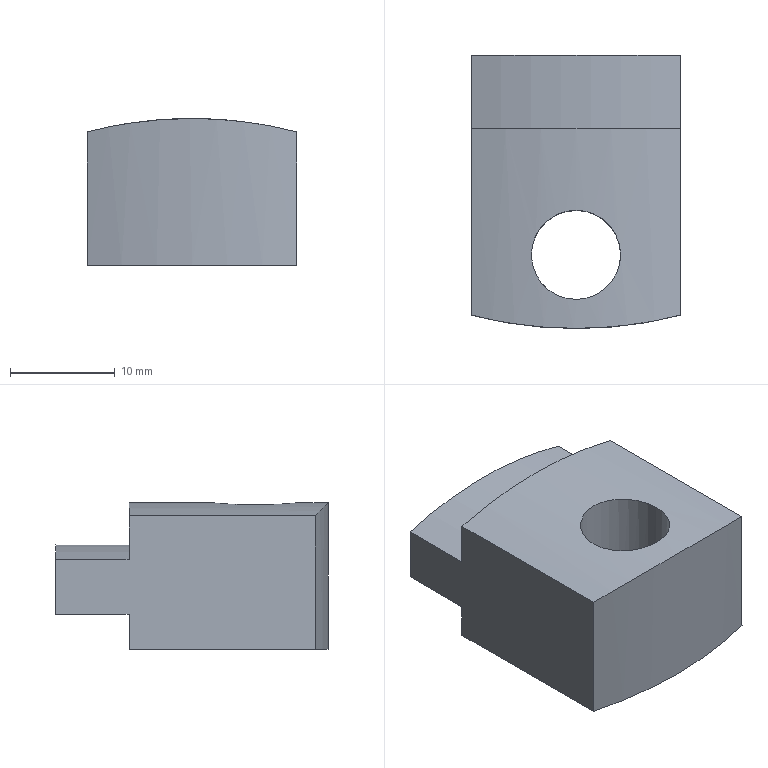Part | NX | features DATUM_CSYS 4, EXTRUDE 3, SKETCH 3 | 1 solid | 11 faces | box 20 x 26 x 14 mm | volume 4969 mm3 | plane 6 | cylinder 5 | commonest cylinder face diameters 80 x2 8.5 x1 62 x1 72 x1
STEP:
#1=CARTESIAN_POINT('',(10.,-21.,-3.657));
#2=VERTEX_POINT('',#1);
#3=CARTESIAN_POINT('',(-10.,-21.,-3.657));
#4=VERTEX_POINT('',#3);
#5=CARTESIAN_POINT('',(0.,-21.,-33.));
#6=DIRECTION('',(0.,-1.,0.));
#7=DIRECTION('',(-1.,0.,0.));
#8=AXIS2_PLACEMENT_3D('',#5,#6,#7);
#9=CIRCLE('',#8,31.);
#10=EDGE_CURVE('',#2,#4,#9,.T.);
#11=ORIENTED_EDGE('',*,*,#10,.F.);
#12=CARTESIAN_POINT('',(10.,-21.,-7.));
#13=VERTEX_POINT('',#12);
#14=CARTESIAN_POINT('',(10.,-21.,7.));
#15=DIRECTION('',(0.,0.,-1.));
#16=VECTOR('',#15,1000.);
#17=LINE('',#14,#16);
#18=EDGE_CURVE('',#2,#13,#17,.T.);
#19=ORIENTED_EDGE('',*,*,#18,.T.);
#20=CARTESIAN_POINT('',(-10.,-21.,-7.));
#21=VERTEX_POINT('',#20);
#22=CARTESIAN_POINT('',(10.,-21.,-7.));
#23=DIRECTION('',(-1.,0.,0.));
#24=VECTOR('',#23,1000.);
#25=LINE('',#22,#24);
#26=EDGE_CURVE('',#13,#21,#25,.T.);
#27=ORIENTED_EDGE('',*,*,#26,.T.);
#28=CARTESIAN_POINT('',(-10.,-21.,7.));
#29=DIRECTION('',(0.,0.,-1.));
#30=VECTOR('',#29,1000.);
#31=LINE('',#28,#30);
#32=EDGE_CURVE('',#4,#21,#31,.T.);
#33=ORIENTED_EDGE('',*,*,#32,.F.);
#34=EDGE_LOOP('',(#11,#19,#27,#33));
#35=FACE_BOUND('',#34,.T.);
#36=CARTESIAN_POINT('',(10.,-21.,7.));
#37=DIRECTION('',(0.,-1.,0.));
#38=DIRECTION('',(0.,0.,-1.));
#39=AXIS2_PLACEMENT_3D('',#36,#37,#38);
#40=PLANE('',#39);
#41=ADVANCED_FACE('',(#35),#40,.F.);
#42=CARTESIAN_POINT('',(10.,-38.73,5.73));
#43=VERTEX_POINT('',#42);
#44=CARTESIAN_POINT('',(10.,-21.,5.73));
#45=VERTEX_POINT('',#44);
#46=CARTESIAN_POINT('',(10.,-83.,5.73));
#47=DIRECTION('',(0.,1.,0.));
#48=VECTOR('',#47,1000.);
#49=LINE('',#46,#48);
#50=EDGE_CURVE('',#43,#45,#49,.T.);
#51=ORIENTED_EDGE('',*,*,#50,.F.);
#52=CARTESIAN_POINT('',(10.,-38.73,-7.));
#53=VERTEX_POINT('',#52);
#54=CARTESIAN_POINT('',(10.,-38.73,7.));
#55=DIRECTION('',(0.,0.,-1.));
#56=VECTOR('',#55,1000.);
#57=LINE('',#54,#56);
#58=EDGE_CURVE('',#43,#53,#57,.T.);
#59=ORIENTED_EDGE('',*,*,#58,.T.);
#60=CARTESIAN_POINT('',(10.,-38.73,-7.));
#61=DIRECTION('',(0.,1.,0.));
#62=VECTOR('',#61,1000.);
#63=LINE('',#60,#62);
#64=EDGE_CURVE('',#53,#13,#63,.T.);
#65=ORIENTED_EDGE('',*,*,#64,.T.);
#66=ORIENTED_EDGE('',*,*,#18,.F.);
#67=CARTESIAN_POINT('',(10.,-14.,-3.657));
#68=VERTEX_POINT('',#67);
#69=CARTESIAN_POINT('',(10.,-14.,-3.657));
#70=DIRECTION('',(0.,-1.,0.));
#71=VECTOR('',#70,1000.);
#72=LINE('',#69,#71);
#73=EDGE_CURVE('',#68,#2,#72,.T.);
#74=ORIENTED_EDGE('',*,*,#73,.F.);
#75=CARTESIAN_POINT('',(10.,-14.,1.583));
#76=VERTEX_POINT('',#75);
#77=CARTESIAN_POINT('',(10.,-14.,1.583));
#78=DIRECTION('',(0.,0.,-1.));
#79=VECTOR('',#78,1000.);
#80=LINE('',#77,#79);
#81=EDGE_CURVE('',#76,#68,#80,.T.);
#82=ORIENTED_EDGE('',*,*,#81,.F.);
#83=CARTESIAN_POINT('',(10.,-21.,1.583));
#84=VERTEX_POINT('',#83);
#85=CARTESIAN_POINT('',(10.,-14.,1.583));
#86=DIRECTION('',(0.,-1.,0.));
#87=VECTOR('',#86,1000.);
#88=LINE('',#85,#87);
#89=EDGE_CURVE('',#76,#84,#88,.T.);
#90=ORIENTED_EDGE('',*,*,#89,.T.);
#91=CARTESIAN_POINT('',(10.,-21.,7.));
#92=DIRECTION('',(0.,0.,-1.));
#93=VECTOR('',#92,1000.);
#94=LINE('',#91,#93);
#95=EDGE_CURVE('',#45,#84,#94,.T.);
#96=ORIENTED_EDGE('',*,*,#95,.F.);
#97=EDGE_LOOP('',(#51,#59,#65,#66,#74,#82,#90,#96));
#98=FACE_BOUND('',#97,.T.);
#99=CARTESIAN_POINT('',(10.,-38.73,7.));
#100=DIRECTION('',(-1.,0.,0.));
#101=DIRECTION('',(0.,0.,1.));
#102=AXIS2_PLACEMENT_3D('',#99,#100,#101);
#103=PLANE('',#102);
#104=ADVANCED_FACE('',(#98),#103,.F.);
#105=CARTESIAN_POINT('',(-10.,-38.73,5.73));
#106=VERTEX_POINT('',#105);
#107=CARTESIAN_POINT('',(0.,0.,-33.));
#108=DIRECTION('',(0.,-0.7071,-0.7071));
#109=DIRECTION('',(0.,0.7071,-0.7071));
#110=AXIS2_PLACEMENT_3D('',#107,#108,#109);
#111=ELLIPSE('',#110,56.569,40.);
#112=EDGE_CURVE('',#106,#43,#111,.F.);
#113=ORIENTED_EDGE('',*,*,#112,.F.);
#114=CARTESIAN_POINT('',(-10.,-38.73,-7.));
#115=VERTEX_POINT('',#114);
#116=CARTESIAN_POINT('',(-10.,-38.73,7.));
#117=DIRECTION('',(0.,0.,-1.));
#118=VECTOR('',#117,1000.);
#119=LINE('',#116,#118);
#120=EDGE_CURVE('',#106,#115,#119,.T.);
#121=ORIENTED_EDGE('',*,*,#120,.T.);
#122=CARTESIAN_POINT('',(0.,0.,-7.));
#123=DIRECTION('',(0.,0.,1.));
#124=DIRECTION('',(1.,0.,0.));
#125=AXIS2_PLACEMENT_3D('',#122,#123,#124);
#126=CIRCLE('',#125,40.);
#127=EDGE_CURVE('',#115,#53,#126,.T.);
#128=ORIENTED_EDGE('',*,*,#127,.T.);
#129=ORIENTED_EDGE('',*,*,#58,.F.);
#130=EDGE_LOOP('',(#113,#121,#128,#129));
#131=FACE_BOUND('',#130,.T.);
#132=CARTESIAN_POINT('',(0.,0.,7.));
#133=DIRECTION('',(0.,0.,-1.));
#134=DIRECTION('',(-1.,0.,0.));
#135=AXIS2_PLACEMENT_3D('',#132,#133,#134);
#136=CYLINDRICAL_SURFACE('',#135,40.);
#137=ADVANCED_FACE('',(#131),#136,.T.);
#138=CARTESIAN_POINT('',(-10.,-21.,1.583));
#139=VERTEX_POINT('',#138);
#140=CARTESIAN_POINT('',(0.,-21.,-33.));
#141=DIRECTION('',(0.,1.,0.));
#142=DIRECTION('',(-1.,0.,0.));
#143=AXIS2_PLACEMENT_3D('',#140,#141,#142);
#144=CIRCLE('',#143,36.);
#145=EDGE_CURVE('',#139,#84,#144,.T.);
#146=ORIENTED_EDGE('',*,*,#145,.F.);
#147=CARTESIAN_POINT('',(-10.,-21.,5.73));
#148=VERTEX_POINT('',#147);
#149=CARTESIAN_POINT('',(-10.,-21.,7.));
#150=DIRECTION('',(0.,0.,-1.));
#151=VECTOR('',#150,1000.);
#152=LINE('',#149,#151);
#153=EDGE_CURVE('',#148,#139,#152,.T.);
#154=ORIENTED_EDGE('',*,*,#153,.F.);
#155=CARTESIAN_POINT('',(0.,-21.,-33.));
#156=DIRECTION('',(0.,-1.,0.));
#157=DIRECTION('',(0.,0.,-1.));
#158=AXIS2_PLACEMENT_3D('',#155,#156,#157);
#159=CIRCLE('',#158,40.);
#160=EDGE_CURVE('',#45,#148,#159,.T.);
#161=ORIENTED_EDGE('',*,*,#160,.F.);
#162=ORIENTED_EDGE('',*,*,#95,.T.);
#163=EDGE_LOOP('',(#146,#154,#161,#162));
#164=FACE_BOUND('',#163,.T.);
#165=CARTESIAN_POINT('',(10.,-21.,7.));
#166=DIRECTION('',(0.,-1.,0.));
#167=DIRECTION('',(0.,0.,-1.));
#168=AXIS2_PLACEMENT_3D('',#165,#166,#167);
#169=PLANE('',#168);
#170=ADVANCED_FACE('',(#164),#169,.F.);
#171=CARTESIAN_POINT('',(4.25,-33.,-7.));
#172=VERTEX_POINT('',#171);
#173=CARTESIAN_POINT('',(0.,-33.,-7.));
#174=DIRECTION('',(0.,0.,1.));
#175=DIRECTION('',(1.,0.,0.));
#176=AXIS2_PLACEMENT_3D('',#173,#174,#175);
#177=CIRCLE('',#176,4.25);
#178=EDGE_CURVE('',#172,#172,#177,.T.);
#179=ORIENTED_EDGE('',*,*,#178,.F.);
#180=EDGE_LOOP('',(#179));
#181=FACE_BOUND('',#180,.T.);
#182=CARTESIAN_POINT('',(0.,-28.75,7.));
#183=VERTEX_POINT('',#182);
#184=CARTESIAN_POINT('',(3.334,-29.672,6.887));
#185=CARTESIAN_POINT('',(-0.0008317,-28.289,7.057));
#186=CARTESIAN_POINT('',(-3.331,-29.671,6.887));
#187=CARTESIAN_POINT('',(-4.709,-32.996,6.717));
#188=CARTESIAN_POINT('',(-3.332,-36.33,6.887));
#189=CARTESIAN_POINT('',(-0.0008624,-37.709,7.056));
#190=CARTESIAN_POINT('',(3.326,-36.334,6.887));
#191=CARTESIAN_POINT('',(4.71,-33.004,6.717));
#192=CARTESIAN_POINT('',(3.334,-29.672,6.887));
#193=CARTESIAN_POINT('',(-0.0008317,-28.289,7.057));
#194=CARTESIAN_POINT('',(-3.331,-29.671,6.887));
#195=B_SPLINE_CURVE_WITH_KNOTS('',3,(#184,#185,#186,#187,#188,#189,#190,#191,#192,#193,#194),.UNSPECIFIED.,.T.,.F.,(1,1,1,1,1,1,1,1,1,1,1,1,1,1,1),(-0.009971,-0.006648,-0.003324,0.,0.003324,0.006648,0.009971,0.0133,0.01662,0.01994,0.02327,0.02659,0.02991,0.03324,0.03656),.UNSPECIFIED.);
#196=EDGE_CURVE('',#183,#183,#195,.T.);
#197=ORIENTED_EDGE('',*,*,#196,.T.);
#198=EDGE_LOOP('',(#197));
#199=FACE_BOUND('',#198,.T.);
#200=CARTESIAN_POINT('',(0.,-33.,7.));
#201=DIRECTION('',(0.,0.,-1.));
#202=DIRECTION('',(-1.,0.,0.));
#203=AXIS2_PLACEMENT_3D('',#200,#201,#202);
#204=CYLINDRICAL_SURFACE('',#203,4.25);
#205=ADVANCED_FACE('',(#181,#199),#204,.F.);
#206=ORIENTED_EDGE('',*,*,#120,.F.);
#207=CARTESIAN_POINT('',(-10.,-83.,5.73));
#208=DIRECTION('',(0.,1.,0.));
#209=VECTOR('',#208,1000.);
#210=LINE('',#207,#209);
#211=EDGE_CURVE('',#106,#148,#210,.T.);
#212=ORIENTED_EDGE('',*,*,#211,.T.);
#213=ORIENTED_EDGE('',*,*,#153,.T.);
#214=CARTESIAN_POINT('',(-10.,-14.,1.583));
#215=VERTEX_POINT('',#214);
#216=CARTESIAN_POINT('',(-10.,-14.,1.583));
#217=DIRECTION('',(0.,-1.,0.));
#218=VECTOR('',#217,1000.);
#219=LINE('',#216,#218);
#220=EDGE_CURVE('',#215,#139,#219,.T.);
#221=ORIENTED_EDGE('',*,*,#220,.F.);
#222=CARTESIAN_POINT('',(-10.,-14.,-3.657));
#223=VERTEX_POINT('',#222);
#224=CARTESIAN_POINT('',(-10.,-14.,-3.657));
#225=DIRECTION('',(0.,0.,1.));
#226=VECTOR('',#225,1000.);
#227=LINE('',#224,#226);
#228=EDGE_CURVE('',#223,#215,#227,.T.);
#229=ORIENTED_EDGE('',*,*,#228,.F.);
#230=CARTESIAN_POINT('',(-10.,-14.,-3.657));
#231=DIRECTION('',(0.,-1.,0.));
#232=VECTOR('',#231,1000.);
#233=LINE('',#230,#232);
#234=EDGE_CURVE('',#223,#4,#233,.T.);
#235=ORIENTED_EDGE('',*,*,#234,.T.);
#236=ORIENTED_EDGE('',*,*,#32,.T.);
#237=CARTESIAN_POINT('',(-10.,-21.,-7.));
#238=DIRECTION('',(0.,-1.,0.));
#239=VECTOR('',#238,1000.);
#240=LINE('',#237,#239);
#241=EDGE_CURVE('',#21,#115,#240,.T.);
#242=ORIENTED_EDGE('',*,*,#241,.T.);
#243=EDGE_LOOP('',(#206,#212,#213,#221,#229,#235,#236,#242));
#244=FACE_BOUND('',#243,.T.);
#245=CARTESIAN_POINT('',(-10.,-21.,7.));
#246=DIRECTION('',(1.,0.,0.));
#247=DIRECTION('',(0.,0.,-1.));
#248=AXIS2_PLACEMENT_3D('',#245,#246,#247);
#249=PLANE('',#248);
#250=ADVANCED_FACE('',(#244),#249,.F.);
#251=ORIENTED_EDGE('',*,*,#241,.F.);
#252=ORIENTED_EDGE('',*,*,#26,.F.);
#253=ORIENTED_EDGE('',*,*,#64,.F.);
#254=ORIENTED_EDGE('',*,*,#127,.F.);
#255=EDGE_LOOP('',(#251,#252,#253,#254));
#256=FACE_BOUND('',#255,.T.);
#257=ORIENTED_EDGE('',*,*,#178,.T.);
#258=EDGE_LOOP('',(#257));
#259=FACE_BOUND('',#258,.T.);
#260=CARTESIAN_POINT('',(0.,0.,-7.));
#261=DIRECTION('',(0.,0.,1.));
#262=DIRECTION('',(1.,0.,0.));
#263=AXIS2_PLACEMENT_3D('',#260,#261,#262);
#264=PLANE('',#263);
#265=ADVANCED_FACE('',(#256,#259),#264,.F.);
#266=ORIENTED_EDGE('',*,*,#196,.F.);
#267=EDGE_LOOP('',(#266));
#268=FACE_BOUND('',#267,.T.);
#269=ORIENTED_EDGE('',*,*,#112,.T.);
#270=ORIENTED_EDGE('',*,*,#50,.T.);
#271=ORIENTED_EDGE('',*,*,#160,.T.);
#272=ORIENTED_EDGE('',*,*,#211,.F.);
#273=EDGE_LOOP('',(#269,#270,#271,#272));
#274=FACE_BOUND('',#273,.T.);
#275=CARTESIAN_POINT('',(0.,-83.,-33.));
#276=DIRECTION('',(0.,1.,0.));
#277=DIRECTION('',(0.,0.,1.));
#278=AXIS2_PLACEMENT_3D('',#275,#276,#277);
#279=CYLINDRICAL_SURFACE('',#278,40.);
#280=ADVANCED_FACE('',(#268,#274),#279,.T.);
#281=ORIENTED_EDGE('',*,*,#145,.T.);
#282=ORIENTED_EDGE('',*,*,#89,.F.);
#283=CARTESIAN_POINT('',(0.,-14.,-33.));
#284=DIRECTION('',(0.,1.,0.));
#285=DIRECTION('',(-1.,0.,0.));
#286=AXIS2_PLACEMENT_3D('',#283,#284,#285);
#287=CIRCLE('',#286,36.);
#288=EDGE_CURVE('',#215,#76,#287,.T.);
#289=ORIENTED_EDGE('',*,*,#288,.F.);
#290=ORIENTED_EDGE('',*,*,#220,.T.);
#291=EDGE_LOOP('',(#281,#282,#289,#290));
#292=FACE_BOUND('',#291,.T.);
#293=CARTESIAN_POINT('',(0.,-14.,-33.));
#294=DIRECTION('',(0.,-1.,0.));
#295=DIRECTION('',(0.,0.,-1.));
#296=AXIS2_PLACEMENT_3D('',#293,#294,#295);
#297=CYLINDRICAL_SURFACE('',#296,36.);
#298=ADVANCED_FACE('',(#292),#297,.T.);
#299=ORIENTED_EDGE('',*,*,#10,.T.);
#300=ORIENTED_EDGE('',*,*,#234,.F.);
#301=CARTESIAN_POINT('',(0.,-14.,-33.));
#302=DIRECTION('',(0.,-1.,0.));
#303=DIRECTION('',(-1.,0.,0.));
#304=AXIS2_PLACEMENT_3D('',#301,#302,#303);
#305=CIRCLE('',#304,31.);
#306=EDGE_CURVE('',#68,#223,#305,.T.);
#307=ORIENTED_EDGE('',*,*,#306,.F.);
#308=ORIENTED_EDGE('',*,*,#73,.T.);
#309=EDGE_LOOP('',(#299,#300,#307,#308));
#310=FACE_BOUND('',#309,.T.);
#311=CARTESIAN_POINT('',(0.,-14.,-33.));
#312=DIRECTION('',(0.,-1.,0.));
#313=DIRECTION('',(0.,0.,-1.));
#314=AXIS2_PLACEMENT_3D('',#311,#312,#313);
#315=CYLINDRICAL_SURFACE('',#314,31.);
#316=ADVANCED_FACE('',(#310),#315,.F.);
#317=ORIENTED_EDGE('',*,*,#228,.T.);
#318=ORIENTED_EDGE('',*,*,#288,.T.);
#319=ORIENTED_EDGE('',*,*,#81,.T.);
#320=ORIENTED_EDGE('',*,*,#306,.T.);
#321=EDGE_LOOP('',(#317,#318,#319,#320));
#322=FACE_BOUND('',#321,.T.);
#323=CARTESIAN_POINT('',(0.,-14.,-33.));
#324=DIRECTION('',(0.,1.,0.));
#325=DIRECTION('',(0.,0.,1.));
#326=AXIS2_PLACEMENT_3D('',#323,#324,#325);
#327=PLANE('',#326);
#328=ADVANCED_FACE('',(#322),#327,.T.);
#329=CLOSED_SHELL('',(#41,#104,#137,#170,#205,#250,#265,#280,#298,#316,#328));
#330=MANIFOLD_SOLID_BREP('',#329);
#331=(LENGTH_UNIT()NAMED_UNIT(*)SI_UNIT(.MILLI.,.METRE.));
#332=UNCERTAINTY_MEASURE_WITH_UNIT(LENGTH_MEASURE(0.0508),#331,'','');
#333=(NAMED_UNIT(*)PLANE_ANGLE_UNIT()SI_UNIT($,.RADIAN.));
#334=(NAMED_UNIT(*)SI_UNIT($,.STERADIAN.)SOLID_ANGLE_UNIT());
#335=(GEOMETRIC_REPRESENTATION_CONTEXT(3)GLOBAL_UNCERTAINTY_ASSIGNED_CONTEXT((#332))GLOBAL_UNIT_ASSIGNED_CONTEXT((#331,#333,#334))REPRESENTATION_CONTEXT('',''));
#336=ADVANCED_BREP_SHAPE_REPRESENTATION('',(#330),#335);